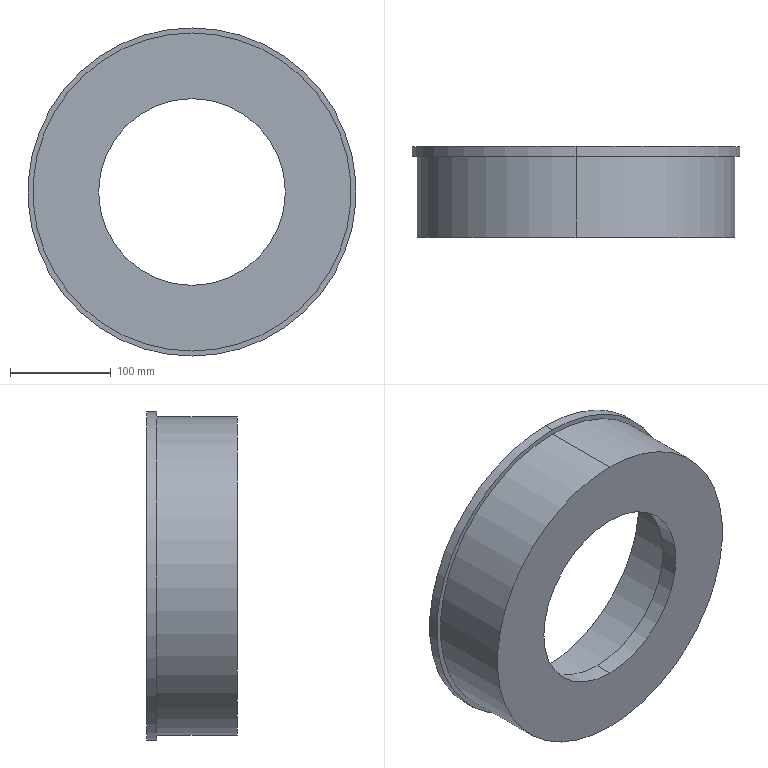Part | SolidWorks | features BaseBody 1 | 1 solid | 12 faces | box 325 x 90 x 325 mm | volume 2757533 mm3 | cylinder 8 | plane 4 | commonest cylinder face diameters 185 x2 260 x2 315 x2 325 x2
STEP:
#1=CARTESIAN_POINT('',(0.,80.,-157.5));
#2=VERTEX_POINT('',#1);
#3=CARTESIAN_POINT('',(0.,80.,157.5));
#4=VERTEX_POINT('',#3);
#5=CARTESIAN_POINT('',(0.,80.,0.));
#6=DIRECTION('',(0.,-1.,0.));
#7=DIRECTION('',(0.,0.,-1.));
#8=AXIS2_PLACEMENT_3D('',#5,#6,#7);
#9=CIRCLE('',#8,157.5);
#10=EDGE_CURVE('',#2,#4,#9,.T.);
#11=ORIENTED_EDGE('',*,*,#10,.T.);
#12=CARTESIAN_POINT('',(0.,0.,157.5));
#13=VERTEX_POINT('',#12);
#14=CARTESIAN_POINT('',(0.,80.,157.5));
#15=DIRECTION('',(0.,-1.,0.));
#16=VECTOR('',#15,1000.);
#17=LINE('',#14,#16);
#18=EDGE_CURVE('',#4,#13,#17,.T.);
#19=ORIENTED_EDGE('',*,*,#18,.T.);
#20=CARTESIAN_POINT('',(0.,0.,-157.5));
#21=VERTEX_POINT('',#20);
#22=CARTESIAN_POINT('',(0.,0.,0.));
#23=DIRECTION('',(0.,-1.,0.));
#24=DIRECTION('',(0.,0.,-1.));
#25=AXIS2_PLACEMENT_3D('',#22,#23,#24);
#26=CIRCLE('',#25,157.5);
#27=EDGE_CURVE('',#21,#13,#26,.T.);
#28=ORIENTED_EDGE('',*,*,#27,.F.);
#29=CARTESIAN_POINT('',(0.,80.,-157.5));
#30=DIRECTION('',(0.,-1.,0.));
#31=VECTOR('',#30,1000.);
#32=LINE('',#29,#31);
#33=EDGE_CURVE('',#2,#21,#32,.T.);
#34=ORIENTED_EDGE('',*,*,#33,.F.);
#35=EDGE_LOOP('',(#11,#19,#28,#34));
#36=FACE_OUTER_BOUND('',#35,.T.);
#37=CARTESIAN_POINT('',(0.,80.,0.));
#38=DIRECTION('',(0.,-1.,0.));
#39=DIRECTION('',(0.,0.,-1.));
#40=AXIS2_PLACEMENT_3D('',#37,#38,#39);
#41=CYLINDRICAL_SURFACE('',#40,157.5);
#42=ADVANCED_FACE('',(#36),#41,.T.);
#43=CARTESIAN_POINT('',(0.,0.,-92.5));
#44=VERTEX_POINT('',#43);
#45=CARTESIAN_POINT('',(0.,0.,92.5));
#46=VERTEX_POINT('',#45);
#47=CARTESIAN_POINT('',(0.,0.,0.));
#48=DIRECTION('',(0.,1.,0.));
#49=DIRECTION('',(0.,0.,1.));
#50=AXIS2_PLACEMENT_3D('',#47,#48,#49);
#51=CIRCLE('',#50,92.5);
#52=EDGE_CURVE('',#44,#46,#51,.T.);
#53=ORIENTED_EDGE('',*,*,#52,.F.);
#54=CARTESIAN_POINT('',(0.,18.,-92.5));
#55=VERTEX_POINT('',#54);
#56=CARTESIAN_POINT('',(0.,0.,-92.5));
#57=DIRECTION('',(0.,1.,0.));
#58=VECTOR('',#57,1000.);
#59=LINE('',#56,#58);
#60=EDGE_CURVE('',#44,#55,#59,.T.);
#61=ORIENTED_EDGE('',*,*,#60,.T.);
#62=CARTESIAN_POINT('',(0.,18.,92.5));
#63=VERTEX_POINT('',#62);
#64=CARTESIAN_POINT('',(0.,18.,0.));
#65=DIRECTION('',(0.,1.,0.));
#66=DIRECTION('',(0.,0.,1.));
#67=AXIS2_PLACEMENT_3D('',#64,#65,#66);
#68=CIRCLE('',#67,92.5);
#69=EDGE_CURVE('',#55,#63,#68,.T.);
#70=ORIENTED_EDGE('',*,*,#69,.T.);
#71=CARTESIAN_POINT('',(0.,0.,92.5));
#72=DIRECTION('',(0.,1.,0.));
#73=VECTOR('',#72,1000.);
#74=LINE('',#71,#73);
#75=EDGE_CURVE('',#46,#63,#74,.T.);
#76=ORIENTED_EDGE('',*,*,#75,.F.);
#77=EDGE_LOOP('',(#53,#61,#70,#76));
#78=FACE_OUTER_BOUND('',#77,.T.);
#79=CARTESIAN_POINT('',(0.,0.,0.));
#80=DIRECTION('',(0.,1.,0.));
#81=DIRECTION('',(0.,0.,1.));
#82=AXIS2_PLACEMENT_3D('',#79,#80,#81);
#83=CYLINDRICAL_SURFACE('',#82,92.5);
#84=ADVANCED_FACE('',(#78),#83,.F.);
#85=CARTESIAN_POINT('',(0.,18.,-130.));
#86=VERTEX_POINT('',#85);
#87=CARTESIAN_POINT('',(0.,18.,130.));
#88=VERTEX_POINT('',#87);
#89=CARTESIAN_POINT('',(0.,18.,0.));
#90=DIRECTION('',(0.,1.,0.));
#91=DIRECTION('',(0.,0.,1.));
#92=AXIS2_PLACEMENT_3D('',#89,#90,#91);
#93=CIRCLE('',#92,130.);
#94=EDGE_CURVE('',#86,#88,#93,.T.);
#95=ORIENTED_EDGE('',*,*,#94,.F.);
#96=CARTESIAN_POINT('',(0.,90.,-130.));
#97=VERTEX_POINT('',#96);
#98=CARTESIAN_POINT('',(0.,18.,-130.));
#99=DIRECTION('',(0.,1.,0.));
#100=VECTOR('',#99,1000.);
#101=LINE('',#98,#100);
#102=EDGE_CURVE('',#86,#97,#101,.T.);
#103=ORIENTED_EDGE('',*,*,#102,.T.);
#104=CARTESIAN_POINT('',(0.,90.,130.));
#105=VERTEX_POINT('',#104);
#106=CARTESIAN_POINT('',(0.,90.,0.));
#107=DIRECTION('',(0.,1.,0.));
#108=DIRECTION('',(0.,0.,1.));
#109=AXIS2_PLACEMENT_3D('',#106,#107,#108);
#110=CIRCLE('',#109,130.);
#111=EDGE_CURVE('',#97,#105,#110,.T.);
#112=ORIENTED_EDGE('',*,*,#111,.T.);
#113=CARTESIAN_POINT('',(0.,18.,130.));
#114=DIRECTION('',(0.,1.,0.));
#115=VECTOR('',#114,1000.);
#116=LINE('',#113,#115);
#117=EDGE_CURVE('',#88,#105,#116,.T.);
#118=ORIENTED_EDGE('',*,*,#117,.F.);
#119=EDGE_LOOP('',(#95,#103,#112,#118));
#120=FACE_OUTER_BOUND('',#119,.T.);
#121=CARTESIAN_POINT('',(0.,18.,0.));
#122=DIRECTION('',(0.,1.,0.));
#123=DIRECTION('',(0.,0.,1.));
#124=AXIS2_PLACEMENT_3D('',#121,#122,#123);
#125=CYLINDRICAL_SURFACE('',#124,130.);
#126=ADVANCED_FACE('',(#120),#125,.F.);
#127=CARTESIAN_POINT('',(0.,90.,162.5));
#128=VERTEX_POINT('',#127);
#129=CARTESIAN_POINT('',(0.,90.,-162.5));
#130=VERTEX_POINT('',#129);
#131=CARTESIAN_POINT('',(0.,90.,0.));
#132=DIRECTION('',(0.,1.,0.));
#133=DIRECTION('',(0.,0.,1.));
#134=AXIS2_PLACEMENT_3D('',#131,#132,#133);
#135=CIRCLE('',#134,162.5);
#136=EDGE_CURVE('',#128,#130,#135,.T.);
#137=ORIENTED_EDGE('',*,*,#136,.F.);
#138=CARTESIAN_POINT('',(0.,80.,162.5));
#139=VERTEX_POINT('',#138);
#140=CARTESIAN_POINT('',(0.,90.,162.5));
#141=DIRECTION('',(0.,-1.,0.));
#142=VECTOR('',#141,1000.);
#143=LINE('',#140,#142);
#144=EDGE_CURVE('',#128,#139,#143,.T.);
#145=ORIENTED_EDGE('',*,*,#144,.T.);
#146=CARTESIAN_POINT('',(0.,80.,-162.5));
#147=VERTEX_POINT('',#146);
#148=CARTESIAN_POINT('',(0.,80.,0.));
#149=DIRECTION('',(0.,-1.,0.));
#150=DIRECTION('',(0.,0.,-1.));
#151=AXIS2_PLACEMENT_3D('',#148,#149,#150);
#152=CIRCLE('',#151,162.5);
#153=EDGE_CURVE('',#147,#139,#152,.T.);
#154=ORIENTED_EDGE('',*,*,#153,.F.);
#155=CARTESIAN_POINT('',(0.,90.,-162.5));
#156=DIRECTION('',(0.,-1.,0.));
#157=VECTOR('',#156,1000.);
#158=LINE('',#155,#157);
#159=EDGE_CURVE('',#130,#147,#158,.T.);
#160=ORIENTED_EDGE('',*,*,#159,.F.);
#161=EDGE_LOOP('',(#137,#145,#154,#160));
#162=FACE_OUTER_BOUND('',#161,.T.);
#163=CARTESIAN_POINT('',(0.,90.,0.));
#164=DIRECTION('',(0.,-1.,0.));
#165=DIRECTION('',(0.,0.,-1.));
#166=AXIS2_PLACEMENT_3D('',#163,#164,#165);
#167=CYLINDRICAL_SURFACE('',#166,162.5);
#168=ADVANCED_FACE('',(#162),#167,.T.);
#169=ORIENTED_EDGE('',*,*,#144,.F.);
#170=CARTESIAN_POINT('',(0.,90.,0.));
#171=DIRECTION('',(0.,1.,0.));
#172=DIRECTION('',(0.,0.,1.));
#173=AXIS2_PLACEMENT_3D('',#170,#171,#172);
#174=CIRCLE('',#173,162.5);
#175=EDGE_CURVE('',#130,#128,#174,.T.);
#176=ORIENTED_EDGE('',*,*,#175,.F.);
#177=ORIENTED_EDGE('',*,*,#159,.T.);
#178=CARTESIAN_POINT('',(0.,80.,0.));
#179=DIRECTION('',(0.,-1.,0.));
#180=DIRECTION('',(0.,0.,-1.));
#181=AXIS2_PLACEMENT_3D('',#178,#179,#180);
#182=CIRCLE('',#181,162.5);
#183=EDGE_CURVE('',#139,#147,#182,.T.);
#184=ORIENTED_EDGE('',*,*,#183,.F.);
#185=EDGE_LOOP('',(#169,#176,#177,#184));
#186=FACE_OUTER_BOUND('',#185,.T.);
#187=CARTESIAN_POINT('',(0.,90.,0.));
#188=DIRECTION('',(0.,-1.,0.));
#189=DIRECTION('',(0.,0.,-1.));
#190=AXIS2_PLACEMENT_3D('',#187,#188,#189);
#191=CYLINDRICAL_SURFACE('',#190,162.5);
#192=ADVANCED_FACE('',(#186),#191,.T.);
#193=CARTESIAN_POINT('',(0.,0.,0.));
#194=DIRECTION('',(0.,1.,0.));
#195=DIRECTION('',(0.,0.,1.));
#196=AXIS2_PLACEMENT_3D('',#193,#194,#195);
#197=CIRCLE('',#196,92.5);
#198=EDGE_CURVE('',#46,#44,#197,.T.);
#199=ORIENTED_EDGE('',*,*,#198,.T.);
#200=ORIENTED_EDGE('',*,*,#52,.T.);
#201=EDGE_LOOP('',(#199,#200));
#202=FACE_BOUND('',#201,.T.);
#203=ORIENTED_EDGE('',*,*,#27,.T.);
#204=CARTESIAN_POINT('',(0.,0.,0.));
#205=DIRECTION('',(0.,-1.,0.));
#206=DIRECTION('',(0.,0.,-1.));
#207=AXIS2_PLACEMENT_3D('',#204,#205,#206);
#208=CIRCLE('',#207,157.5);
#209=EDGE_CURVE('',#13,#21,#208,.T.);
#210=ORIENTED_EDGE('',*,*,#209,.T.);
#211=EDGE_LOOP('',(#203,#210));
#212=FACE_OUTER_BOUND('',#211,.T.);
#213=CARTESIAN_POINT('',(0.,0.,0.));
#214=DIRECTION('',(0.,1.,0.));
#215=DIRECTION('',(0.,0.,1.));
#216=AXIS2_PLACEMENT_3D('',#213,#214,#215);
#217=PLANE('',#216);
#218=ADVANCED_FACE('',(#202,#212),#217,.F.);
#219=CARTESIAN_POINT('',(0.,90.,0.));
#220=DIRECTION('',(0.,1.,0.));
#221=DIRECTION('',(0.,0.,1.));
#222=AXIS2_PLACEMENT_3D('',#219,#220,#221);
#223=CIRCLE('',#222,130.);
#224=EDGE_CURVE('',#105,#97,#223,.T.);
#225=ORIENTED_EDGE('',*,*,#224,.F.);
#226=ORIENTED_EDGE('',*,*,#111,.F.);
#227=EDGE_LOOP('',(#225,#226));
#228=FACE_BOUND('',#227,.T.);
#229=ORIENTED_EDGE('',*,*,#175,.T.);
#230=ORIENTED_EDGE('',*,*,#136,.T.);
#231=EDGE_LOOP('',(#229,#230));
#232=FACE_OUTER_BOUND('',#231,.T.);
#233=CARTESIAN_POINT('',(0.,90.,0.));
#234=DIRECTION('',(0.,1.,0.));
#235=DIRECTION('',(0.,0.,1.));
#236=AXIS2_PLACEMENT_3D('',#233,#234,#235);
#237=PLANE('',#236);
#238=ADVANCED_FACE('',(#228,#232),#237,.T.);
#239=ORIENTED_EDGE('',*,*,#102,.F.);
#240=CARTESIAN_POINT('',(0.,18.,0.));
#241=DIRECTION('',(0.,1.,0.));
#242=DIRECTION('',(0.,0.,1.));
#243=AXIS2_PLACEMENT_3D('',#240,#241,#242);
#244=CIRCLE('',#243,130.);
#245=EDGE_CURVE('',#88,#86,#244,.T.);
#246=ORIENTED_EDGE('',*,*,#245,.F.);
#247=ORIENTED_EDGE('',*,*,#117,.T.);
#248=ORIENTED_EDGE('',*,*,#224,.T.);
#249=EDGE_LOOP('',(#239,#246,#247,#248));
#250=FACE_OUTER_BOUND('',#249,.T.);
#251=CARTESIAN_POINT('',(0.,18.,0.));
#252=DIRECTION('',(0.,1.,0.));
#253=DIRECTION('',(0.,0.,1.));
#254=AXIS2_PLACEMENT_3D('',#251,#252,#253);
#255=CYLINDRICAL_SURFACE('',#254,130.);
#256=ADVANCED_FACE('',(#250),#255,.F.);
#257=CARTESIAN_POINT('',(0.,18.,0.));
#258=DIRECTION('',(0.,1.,0.));
#259=DIRECTION('',(0.,0.,1.));
#260=AXIS2_PLACEMENT_3D('',#257,#258,#259);
#261=CIRCLE('',#260,92.5);
#262=EDGE_CURVE('',#63,#55,#261,.T.);
#263=ORIENTED_EDGE('',*,*,#262,.F.);
#264=ORIENTED_EDGE('',*,*,#69,.F.);
#265=EDGE_LOOP('',(#263,#264));
#266=FACE_BOUND('',#265,.T.);
#267=ORIENTED_EDGE('',*,*,#245,.T.);
#268=ORIENTED_EDGE('',*,*,#94,.T.);
#269=EDGE_LOOP('',(#267,#268));
#270=FACE_OUTER_BOUND('',#269,.T.);
#271=CARTESIAN_POINT('',(0.,18.,0.));
#272=DIRECTION('',(0.,1.,0.));
#273=DIRECTION('',(0.,0.,1.));
#274=AXIS2_PLACEMENT_3D('',#271,#272,#273);
#275=PLANE('',#274);
#276=ADVANCED_FACE('',(#266,#270),#275,.T.);
#277=ORIENTED_EDGE('',*,*,#60,.F.);
#278=ORIENTED_EDGE('',*,*,#198,.F.);
#279=ORIENTED_EDGE('',*,*,#75,.T.);
#280=ORIENTED_EDGE('',*,*,#262,.T.);
#281=EDGE_LOOP('',(#277,#278,#279,#280));
#282=FACE_OUTER_BOUND('',#281,.T.);
#283=CARTESIAN_POINT('',(0.,0.,0.));
#284=DIRECTION('',(0.,1.,0.));
#285=DIRECTION('',(0.,0.,1.));
#286=AXIS2_PLACEMENT_3D('',#283,#284,#285);
#287=CYLINDRICAL_SURFACE('',#286,92.5);
#288=ADVANCED_FACE('',(#282),#287,.F.);
#289=ORIENTED_EDGE('',*,*,#10,.F.);
#290=CARTESIAN_POINT('',(0.,80.,0.));
#291=DIRECTION('',(0.,-1.,0.));
#292=DIRECTION('',(0.,0.,-1.));
#293=AXIS2_PLACEMENT_3D('',#290,#291,#292);
#294=CIRCLE('',#293,157.5);
#295=EDGE_CURVE('',#4,#2,#294,.T.);
#296=ORIENTED_EDGE('',*,*,#295,.F.);
#297=EDGE_LOOP('',(#289,#296));
#298=FACE_BOUND('',#297,.T.);
#299=ORIENTED_EDGE('',*,*,#153,.T.);
#300=ORIENTED_EDGE('',*,*,#183,.T.);
#301=EDGE_LOOP('',(#299,#300));
#302=FACE_OUTER_BOUND('',#301,.T.);
#303=CARTESIAN_POINT('',(0.,80.,0.));
#304=DIRECTION('',(0.,-1.,0.));
#305=DIRECTION('',(0.,0.,-1.));
#306=AXIS2_PLACEMENT_3D('',#303,#304,#305);
#307=PLANE('',#306);
#308=ADVANCED_FACE('',(#298,#302),#307,.T.);
#309=ORIENTED_EDGE('',*,*,#18,.F.);
#310=ORIENTED_EDGE('',*,*,#295,.T.);
#311=ORIENTED_EDGE('',*,*,#33,.T.);
#312=ORIENTED_EDGE('',*,*,#209,.F.);
#313=EDGE_LOOP('',(#309,#310,#311,#312));
#314=FACE_OUTER_BOUND('',#313,.T.);
#315=CARTESIAN_POINT('',(0.,80.,0.));
#316=DIRECTION('',(0.,-1.,0.));
#317=DIRECTION('',(0.,0.,-1.));
#318=AXIS2_PLACEMENT_3D('',#315,#316,#317);
#319=CYLINDRICAL_SURFACE('',#318,157.5);
#320=ADVANCED_FACE('',(#314),#319,.T.);
#321=CLOSED_SHELL('',(#42,#84,#126,#168,#192,#218,#238,#256,#276,#288,#308,#320));
#322=MANIFOLD_SOLID_BREP('',#321);
#323=CARTESIAN_POINT('',(0.,0.,0.));
#324=DIRECTION('',(0.,0.,1.));
#325=DIRECTION('',(1.,0.,0.));
#326=AXIS2_PLACEMENT_3D('',#323,#324,#325);
#327=(LENGTH_UNIT()NAMED_UNIT(*)SI_UNIT(.MILLI.,.METRE.));
#328=UNCERTAINTY_MEASURE_WITH_UNIT(LENGTH_MEASURE(0.00001),#327,'','');
#329=(NAMED_UNIT(*)PLANE_ANGLE_UNIT()SI_UNIT($,.RADIAN.));
#330=(NAMED_UNIT(*)SI_UNIT($,.STERADIAN.)SOLID_ANGLE_UNIT());
#331=(GEOMETRIC_REPRESENTATION_CONTEXT(3)GLOBAL_UNCERTAINTY_ASSIGNED_CONTEXT((#328))GLOBAL_UNIT_ASSIGNED_CONTEXT((#327,#329,#330))REPRESENTATION_CONTEXT('',''));
#332=ADVANCED_BREP_SHAPE_REPRESENTATION('',(#322,#326),#331);